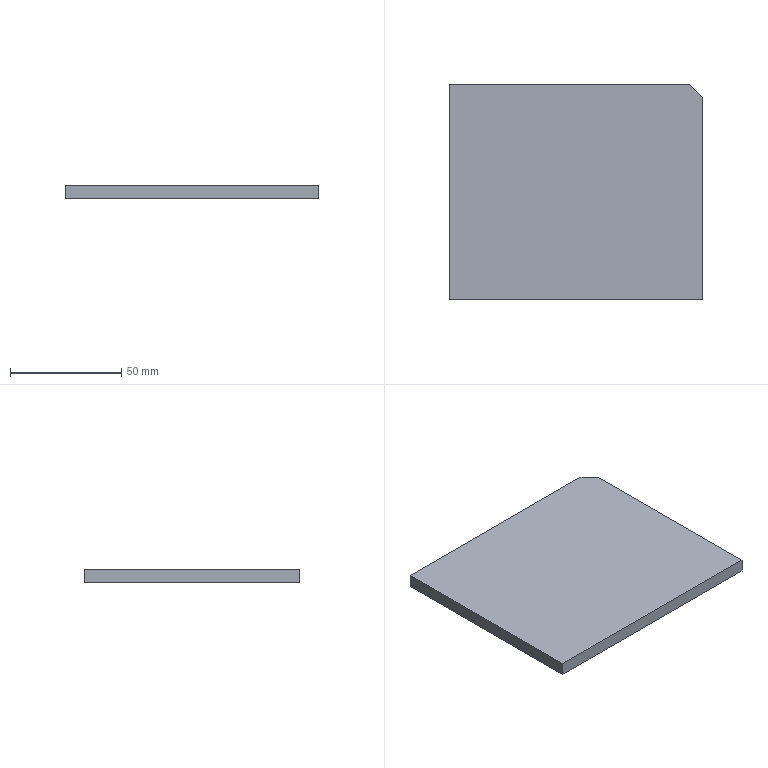Part | STEP file | VD-SYL0380DJ1006_1_1_4-3_VD-SYL | 1 solid | 7 faces | box 114 x 97 x 6 mm | volume 66240 mm3 | plane 7
STEP:
#1=CARTESIAN_POINT('',(-57.,48.5,6.));
#2=VERTEX_POINT('',#1);
#3=CARTESIAN_POINT('',(51.,48.5,6.));
#4=VERTEX_POINT('',#3);
#5=CARTESIAN_POINT('',(-57.,48.5,6.));
#6=DIRECTION('',(1.,0.,0.));
#7=VECTOR('',#6,1000.);
#8=LINE('',#5,#7);
#9=EDGE_CURVE('',#2,#4,#8,.T.);
#10=ORIENTED_EDGE('',*,*,#9,.T.);
#11=CARTESIAN_POINT('',(51.,48.5,0.));
#12=VERTEX_POINT('',#11);
#13=CARTESIAN_POINT('',(51.,48.5,6.));
#14=DIRECTION('',(0.,0.,-1.));
#15=VECTOR('',#14,1000.);
#16=LINE('',#13,#15);
#17=EDGE_CURVE('',#4,#12,#16,.T.);
#18=ORIENTED_EDGE('',*,*,#17,.T.);
#19=CARTESIAN_POINT('',(-57.,48.5,0.));
#20=VERTEX_POINT('',#19);
#21=CARTESIAN_POINT('',(51.,48.5,0.));
#22=DIRECTION('',(-1.,0.,0.));
#23=VECTOR('',#22,1000.);
#24=LINE('',#21,#23);
#25=EDGE_CURVE('',#12,#20,#24,.T.);
#26=ORIENTED_EDGE('',*,*,#25,.T.);
#27=CARTESIAN_POINT('',(-57.,48.5,6.));
#28=DIRECTION('',(0.,0.,-1.));
#29=VECTOR('',#28,1000.);
#30=LINE('',#27,#29);
#31=EDGE_CURVE('',#2,#20,#30,.T.);
#32=ORIENTED_EDGE('',*,*,#31,.F.);
#33=EDGE_LOOP('',(#10,#18,#26,#32));
#34=FACE_OUTER_BOUND('',#33,.T.);
#35=CARTESIAN_POINT('',(0.,48.5,3.));
#36=DIRECTION('',(0.,-1.,0.));
#37=DIRECTION('',(0.,0.,-1.));
#38=AXIS2_PLACEMENT_3D('',#35,#36,#37);
#39=PLANE('',#38);
#40=ADVANCED_FACE('',(#34),#39,.F.);
#41=CARTESIAN_POINT('',(-57.,-48.5,0.));
#42=VERTEX_POINT('',#41);
#43=CARTESIAN_POINT('',(-57.,48.5,0.));
#44=DIRECTION('',(0.,-1.,0.));
#45=VECTOR('',#44,1000.);
#46=LINE('',#43,#45);
#47=EDGE_CURVE('',#20,#42,#46,.T.);
#48=ORIENTED_EDGE('',*,*,#47,.F.);
#49=ORIENTED_EDGE('',*,*,#25,.F.);
#50=CARTESIAN_POINT('',(57.,42.5,0.));
#51=VERTEX_POINT('',#50);
#52=CARTESIAN_POINT('',(51.,48.5,0.));
#53=DIRECTION('',(0.7071,-0.7071,0.));
#54=VECTOR('',#53,1000.);
#55=LINE('',#52,#54);
#56=EDGE_CURVE('',#12,#51,#55,.T.);
#57=ORIENTED_EDGE('',*,*,#56,.T.);
#58=CARTESIAN_POINT('',(57.,-48.5,0.));
#59=VERTEX_POINT('',#58);
#60=CARTESIAN_POINT('',(57.,-48.5,0.));
#61=DIRECTION('',(0.,1.,0.));
#62=VECTOR('',#61,1000.);
#63=LINE('',#60,#62);
#64=EDGE_CURVE('',#59,#51,#63,.T.);
#65=ORIENTED_EDGE('',*,*,#64,.F.);
#66=CARTESIAN_POINT('',(-57.,-48.5,0.));
#67=DIRECTION('',(1.,0.,0.));
#68=VECTOR('',#67,1000.);
#69=LINE('',#66,#68);
#70=EDGE_CURVE('',#42,#59,#69,.T.);
#71=ORIENTED_EDGE('',*,*,#70,.F.);
#72=EDGE_LOOP('',(#48,#49,#57,#65,#71));
#73=FACE_OUTER_BOUND('',#72,.T.);
#74=CARTESIAN_POINT('',(0.,0.,0.));
#75=DIRECTION('',(0.,0.,1.));
#76=DIRECTION('',(1.,0.,0.));
#77=AXIS2_PLACEMENT_3D('',#74,#75,#76);
#78=PLANE('',#77);
#79=ADVANCED_FACE('',(#73),#78,.F.);
#80=ORIENTED_EDGE('',*,*,#31,.T.);
#81=ORIENTED_EDGE('',*,*,#47,.T.);
#82=CARTESIAN_POINT('',(-57.,-48.5,6.));
#83=VERTEX_POINT('',#82);
#84=CARTESIAN_POINT('',(-57.,-48.5,6.));
#85=DIRECTION('',(0.,0.,-1.));
#86=VECTOR('',#85,1000.);
#87=LINE('',#84,#86);
#88=EDGE_CURVE('',#83,#42,#87,.T.);
#89=ORIENTED_EDGE('',*,*,#88,.F.);
#90=CARTESIAN_POINT('',(-57.,-48.5,6.));
#91=DIRECTION('',(0.,1.,0.));
#92=VECTOR('',#91,1000.);
#93=LINE('',#90,#92);
#94=EDGE_CURVE('',#83,#2,#93,.T.);
#95=ORIENTED_EDGE('',*,*,#94,.T.);
#96=EDGE_LOOP('',(#80,#81,#89,#95));
#97=FACE_OUTER_BOUND('',#96,.T.);
#98=CARTESIAN_POINT('',(-57.,0.,3.));
#99=DIRECTION('',(1.,0.,0.));
#100=DIRECTION('',(0.,1.,0.));
#101=AXIS2_PLACEMENT_3D('',#98,#99,#100);
#102=PLANE('',#101);
#103=ADVANCED_FACE('',(#97),#102,.F.);
#104=CARTESIAN_POINT('',(57.,42.5,6.));
#105=VERTEX_POINT('',#104);
#106=CARTESIAN_POINT('',(57.,42.5,6.));
#107=DIRECTION('',(-0.7071,0.7071,0.));
#108=VECTOR('',#107,1000.);
#109=LINE('',#106,#108);
#110=EDGE_CURVE('',#105,#4,#109,.T.);
#111=ORIENTED_EDGE('',*,*,#110,.T.);
#112=ORIENTED_EDGE('',*,*,#9,.F.);
#113=ORIENTED_EDGE('',*,*,#94,.F.);
#114=CARTESIAN_POINT('',(57.,-48.5,6.));
#115=VERTEX_POINT('',#114);
#116=CARTESIAN_POINT('',(57.,-48.5,6.));
#117=DIRECTION('',(-1.,0.,0.));
#118=VECTOR('',#117,1000.);
#119=LINE('',#116,#118);
#120=EDGE_CURVE('',#115,#83,#119,.T.);
#121=ORIENTED_EDGE('',*,*,#120,.F.);
#122=CARTESIAN_POINT('',(57.,42.5,6.));
#123=DIRECTION('',(0.,-1.,0.));
#124=VECTOR('',#123,1000.);
#125=LINE('',#122,#124);
#126=EDGE_CURVE('',#105,#115,#125,.T.);
#127=ORIENTED_EDGE('',*,*,#126,.F.);
#128=EDGE_LOOP('',(#111,#112,#113,#121,#127));
#129=FACE_OUTER_BOUND('',#128,.T.);
#130=CARTESIAN_POINT('',(0.,0.,6.));
#131=DIRECTION('',(0.,0.,1.));
#132=DIRECTION('',(1.,0.,0.));
#133=AXIS2_PLACEMENT_3D('',#130,#131,#132);
#134=PLANE('',#133);
#135=ADVANCED_FACE('',(#129),#134,.T.);
#136=ORIENTED_EDGE('',*,*,#88,.T.);
#137=ORIENTED_EDGE('',*,*,#70,.T.);
#138=CARTESIAN_POINT('',(57.,-48.5,6.));
#139=DIRECTION('',(0.,0.,-1.));
#140=VECTOR('',#139,1000.);
#141=LINE('',#138,#140);
#142=EDGE_CURVE('',#115,#59,#141,.T.);
#143=ORIENTED_EDGE('',*,*,#142,.F.);
#144=ORIENTED_EDGE('',*,*,#120,.T.);
#145=EDGE_LOOP('',(#136,#137,#143,#144));
#146=FACE_OUTER_BOUND('',#145,.T.);
#147=CARTESIAN_POINT('',(0.,-48.5,3.));
#148=DIRECTION('',(0.,1.,0.));
#149=DIRECTION('',(1.,0.,0.));
#150=AXIS2_PLACEMENT_3D('',#147,#148,#149);
#151=PLANE('',#150);
#152=ADVANCED_FACE('',(#146),#151,.F.);
#153=ORIENTED_EDGE('',*,*,#64,.T.);
#154=CARTESIAN_POINT('',(57.,42.5,0.));
#155=DIRECTION('',(0.,0.,1.));
#156=VECTOR('',#155,1000.);
#157=LINE('',#154,#156);
#158=EDGE_CURVE('',#51,#105,#157,.T.);
#159=ORIENTED_EDGE('',*,*,#158,.T.);
#160=ORIENTED_EDGE('',*,*,#126,.T.);
#161=ORIENTED_EDGE('',*,*,#142,.T.);
#162=EDGE_LOOP('',(#153,#159,#160,#161));
#163=FACE_OUTER_BOUND('',#162,.T.);
#164=CARTESIAN_POINT('',(57.,0.,3.));
#165=DIRECTION('',(-1.,0.,0.));
#166=DIRECTION('',(0.,0.,1.));
#167=AXIS2_PLACEMENT_3D('',#164,#165,#166);
#168=PLANE('',#167);
#169=ADVANCED_FACE('',(#163),#168,.F.);
#170=ORIENTED_EDGE('',*,*,#56,.F.);
#171=ORIENTED_EDGE('',*,*,#17,.F.);
#172=ORIENTED_EDGE('',*,*,#110,.F.);
#173=ORIENTED_EDGE('',*,*,#158,.F.);
#174=EDGE_LOOP('',(#170,#171,#172,#173));
#175=FACE_OUTER_BOUND('',#174,.T.);
#176=CARTESIAN_POINT('',(54.,45.5,3.));
#177=DIRECTION('',(0.7071,0.7071,0.));
#178=DIRECTION('',(0.,0.,-1.));
#179=AXIS2_PLACEMENT_3D('',#176,#177,#178);
#180=PLANE('',#179);
#181=ADVANCED_FACE('',(#175),#180,.T.);
#182=CLOSED_SHELL('',(#40,#79,#103,#135,#152,#169,#181));
#183=MANIFOLD_SOLID_BREP('',#182);
#184=CARTESIAN_POINT('',(0.,0.,0.));
#185=DIRECTION('',(0.,0.,1.));
#186=DIRECTION('',(1.,0.,0.));
#187=AXIS2_PLACEMENT_3D('',#184,#185,#186);
#188=(LENGTH_UNIT()NAMED_UNIT(*)SI_UNIT(.MILLI.,.METRE.));
#189=UNCERTAINTY_MEASURE_WITH_UNIT(LENGTH_MEASURE(0.00001),#188,'','');
#190=(NAMED_UNIT(*)PLANE_ANGLE_UNIT()SI_UNIT($,.RADIAN.));
#191=(NAMED_UNIT(*)SI_UNIT($,.STERADIAN.)SOLID_ANGLE_UNIT());
#192=(GEOMETRIC_REPRESENTATION_CONTEXT(3)GLOBAL_UNCERTAINTY_ASSIGNED_CONTEXT((#189))GLOBAL_UNIT_ASSIGNED_CONTEXT((#188,#190,#191))REPRESENTATION_CONTEXT('',''));
#193=ADVANCED_BREP_SHAPE_REPRESENTATION('',(#183,#187),#192);